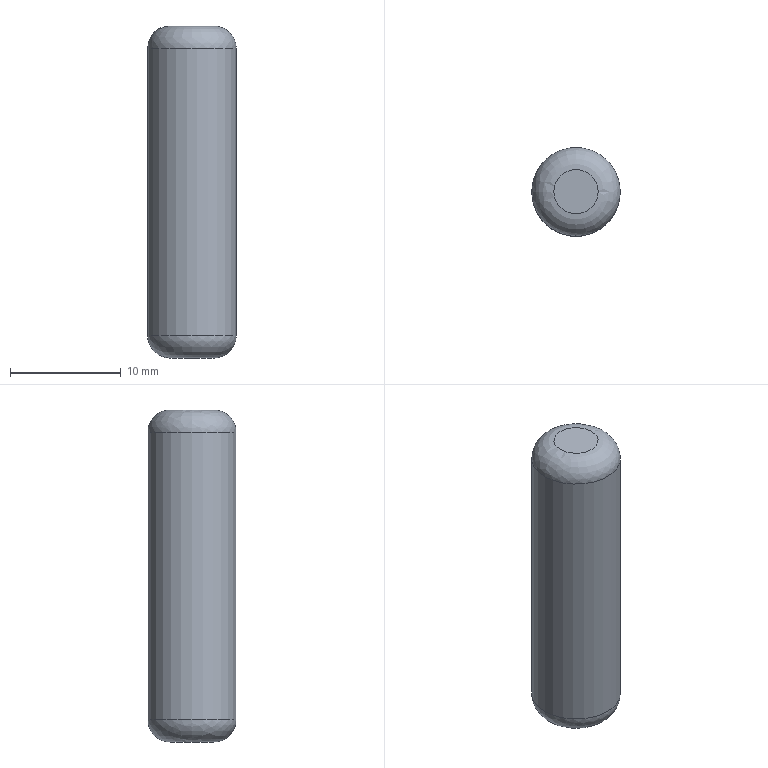Part | STEP file | Tube feed_id1762_x_t | 1 solid | 5 faces | box 8 x 8 x 30 mm | volume 1469 mm3 | plane 2 | spline 2 | cylinder 1 | commonest cylinder face diameters 8 x1
STEP:
#1=CARTESIAN_POINT('',(0.,0.,0.));
#2=DIRECTION('',(0.,0.,1.));
#3=DIRECTION('',(1.,0.,0.));
#4=AXIS2_PLACEMENT_3D('',#1,#2,#3);
#5=CARTESIAN_POINT('',(119.,82.036,-39.5));
#6=VERTEX_POINT('',#5);
#7=CARTESIAN_POINT('',(121.,82.036,-39.5));
#8=DIRECTION('',(0.,0.,-1.));
#9=DIRECTION('',(-1.,0.,0.));
#10=AXIS2_PLACEMENT_3D('',#7,#8,#9);
#11=CIRCLE('',#10,2.);
#12=CARTESIAN_POINT('',(121.,82.036,-39.5));
#13=DIRECTION('',(0.,0.,-1.));
#14=DIRECTION('',(-1.,0.,0.));
#15=AXIS2_PLACEMENT_3D('',#12,#13,#14);
#16=PLANE('',#15);
#17=CARTESIAN_POINT('',(0.,0.));
#18=DIRECTION('',(1.,0.));
#19=AXIS2_PLACEMENT_2D('',#17,#18);
#20=CIRCLE('',#19,2.);
#21=(GEOMETRIC_REPRESENTATION_CONTEXT(2)PARAMETRIC_REPRESENTATION_CONTEXT()REPRESENTATION_CONTEXT('',''));
#22=DEFINITIONAL_REPRESENTATION('',(#20),#21);
#23=PCURVE('',#16,#22);
#24=CARTESIAN_POINT('',(119.,82.036,-39.5));
#25=CARTESIAN_POINT('',(119.,86.036,-39.5));
#26=CARTESIAN_POINT('',(123.,86.036,-39.5));
#27=CARTESIAN_POINT('',(123.,82.036,-39.5));
#28=CARTESIAN_POINT('',(123.,78.036,-39.5));
#29=CARTESIAN_POINT('',(119.,78.036,-39.5));
#30=CARTESIAN_POINT('',(119.,82.036,-39.5));
#31=CARTESIAN_POINT('',(117.828,82.036,-39.5));
#32=CARTESIAN_POINT('',(117.828,88.379,-39.5));
#33=CARTESIAN_POINT('',(124.172,88.379,-39.5));
#34=CARTESIAN_POINT('',(124.172,82.036,-39.5));
#35=CARTESIAN_POINT('',(124.172,75.692,-39.5));
#36=CARTESIAN_POINT('',(117.828,75.692,-39.5));
#37=CARTESIAN_POINT('',(117.828,82.036,-39.5));
#38=CARTESIAN_POINT('',(117.,82.036,-38.672));
#39=CARTESIAN_POINT('',(117.,90.036,-38.672));
#40=CARTESIAN_POINT('',(125.,90.036,-38.672));
#41=CARTESIAN_POINT('',(125.,82.036,-38.672));
#42=CARTESIAN_POINT('',(125.,74.036,-38.672));
#43=CARTESIAN_POINT('',(117.,74.036,-38.672));
#44=CARTESIAN_POINT('',(117.,82.036,-38.672));
#45=CARTESIAN_POINT('',(117.,82.036,-37.5));
#46=CARTESIAN_POINT('',(117.,90.036,-37.5));
#47=CARTESIAN_POINT('',(125.,90.036,-37.5));
#48=CARTESIAN_POINT('',(125.,82.036,-37.5));
#49=CARTESIAN_POINT('',(125.,74.036,-37.5));
#50=CARTESIAN_POINT('',(117.,74.036,-37.5));
#51=CARTESIAN_POINT('',(117.,82.036,-37.5));
#52=(BOUNDED_SURFACE()B_SPLINE_SURFACE(3,3,((#24,#25,#26,#27,#28,#29,#30),(#31,#32,#33,#34,#35,#36,#37),(#38,#39,#40,#41,#42,#43,#44),(#45,#46,#47,#48,#49,#50,#51)),.UNSPECIFIED.,.F.,.T.,.F.)B_SPLINE_SURFACE_WITH_KNOTS((4,4),(1,3,3,3,1),(0.,1.),(-0.5,0.,0.5,1.,1.5),.UNSPECIFIED.)GEOMETRIC_REPRESENTATION_ITEM()RATIONAL_B_SPLINE_SURFACE(((1.,0.3333,0.3333,1.,0.3333,0.3333,1.),(0.8047,0.2682,0.2682,0.8047,0.2682,0.2682,0.8047),(0.8047,0.2682,0.2682,0.8047,0.2682,0.2682,0.8047),(1.,0.3333,0.3333,1.,0.3333,0.3333,1.)))REPRESENTATION_ITEM('')SURFACE());
#53=CARTESIAN_POINT('',(0.,0.));
#54=CARTESIAN_POINT('',(0.,0.02352));
#55=CARTESIAN_POINT('',(0.,0.06491));
#56=CARTESIAN_POINT('',(0.,0.1146));
#57=CARTESIAN_POINT('',(0.,0.1575));
#58=CARTESIAN_POINT('',(0.,0.196));
#59=CARTESIAN_POINT('',(0.,0.2322));
#60=CARTESIAN_POINT('',(0.,0.2678));
#61=CARTESIAN_POINT('',(0.,0.304));
#62=CARTESIAN_POINT('',(0.,0.3425));
#63=CARTESIAN_POINT('',(0.,0.3856));
#64=CARTESIAN_POINT('',(0.,0.4343));
#65=CARTESIAN_POINT('',(0.,0.5));
#66=CARTESIAN_POINT('',(0.,0.5657));
#67=CARTESIAN_POINT('',(0.,0.6144));
#68=CARTESIAN_POINT('',(0.,0.6575));
#69=CARTESIAN_POINT('',(0.,0.696));
#70=CARTESIAN_POINT('',(0.,0.7322));
#71=CARTESIAN_POINT('',(0.,0.7678));
#72=CARTESIAN_POINT('',(0.,0.804));
#73=CARTESIAN_POINT('',(0.,0.8425));
#74=CARTESIAN_POINT('',(0.,0.8854));
#75=CARTESIAN_POINT('',(0.,0.9351));
#76=CARTESIAN_POINT('',(0.,0.9765));
#77=CARTESIAN_POINT('',(0.,1.));
#78=B_SPLINE_CURVE_WITH_KNOTS('',3,(#53,#54,#55,#56,#57,#58,#59,#60,#61,#62,#63,#64,#65,#66,#67,#68,#69,#70,#71,#72,#73,#74,#75,#76,#77),.UNSPECIFIED.,.F.,.F.,(4,1,1,1,1,1,1,1,1,1,1,1,1,1,1,1,1,1,1,1,1,1,4),(0.,0.2856,0.5712,0.8568,1.142,1.428,1.714,1.999,2.285,2.57,2.856,3.142,3.427,3.713,3.998,4.284,4.57,4.855,5.141,5.426,5.712,5.998,6.283),.QUASI_UNIFORM_KNOTS.);
#79=(GEOMETRIC_REPRESENTATION_CONTEXT(2)PARAMETRIC_REPRESENTATION_CONTEXT()REPRESENTATION_CONTEXT('',''));
#80=DEFINITIONAL_REPRESENTATION('',(#78),#79);
#81=PCURVE('',#52,#80);
#82=SURFACE_CURVE('',#11,(#23,#81),.PCURVE_S1.);
#83=EDGE_CURVE('',#6,#6,#82,.T.);
#84=ORIENTED_EDGE('',*,*,#83,.T.);
#85=EDGE_LOOP('',(#84));
#86=FACE_BOUND('',#85,.T.);
#87=ADVANCED_FACE('',(#86),#16,.T.);
#88=CARTESIAN_POINT('',(117.,82.036,-11.5));
#89=VERTEX_POINT('',#88);
#90=CARTESIAN_POINT('',(121.,82.036,-11.5));
#91=DIRECTION('',(0.,0.,-1.));
#92=DIRECTION('',(-1.,0.,0.));
#93=AXIS2_PLACEMENT_3D('',#90,#91,#92);
#94=CIRCLE('',#93,4.);
#95=CARTESIAN_POINT('',(121.,82.036,-39.5));
#96=DIRECTION('',(0.,0.,1.));
#97=DIRECTION('',(1.,0.,0.));
#98=AXIS2_PLACEMENT_3D('',#95,#96,#97);
#99=CYLINDRICAL_SURFACE('',#98,4.);
#100=CARTESIAN_POINT('',(9.425,28.));
#101=DIRECTION('',(-1.,0.));
#102=VECTOR('',#101,1.);
#103=LINE('',#100,#102);
#104=(GEOMETRIC_REPRESENTATION_CONTEXT(2)PARAMETRIC_REPRESENTATION_CONTEXT()REPRESENTATION_CONTEXT('',''));
#105=DEFINITIONAL_REPRESENTATION('',(#103),#104);
#106=PCURVE('',#99,#105);
#107=CARTESIAN_POINT('',(117.,82.036,-11.5));
#108=CARTESIAN_POINT('',(117.,90.036,-11.5));
#109=CARTESIAN_POINT('',(125.,90.036,-11.5));
#110=CARTESIAN_POINT('',(125.,82.036,-11.5));
#111=CARTESIAN_POINT('',(125.,74.036,-11.5));
#112=CARTESIAN_POINT('',(117.,74.036,-11.5));
#113=CARTESIAN_POINT('',(117.,82.036,-11.5));
#114=CARTESIAN_POINT('',(117.,82.036,-10.328));
#115=CARTESIAN_POINT('',(117.,90.036,-10.328));
#116=CARTESIAN_POINT('',(125.,90.036,-10.328));
#117=CARTESIAN_POINT('',(125.,82.036,-10.328));
#118=CARTESIAN_POINT('',(125.,74.036,-10.328));
#119=CARTESIAN_POINT('',(117.,74.036,-10.328));
#120=CARTESIAN_POINT('',(117.,82.036,-10.328));
#121=CARTESIAN_POINT('',(117.828,82.036,-9.5));
#122=CARTESIAN_POINT('',(117.828,88.379,-9.5));
#123=CARTESIAN_POINT('',(124.172,88.379,-9.5));
#124=CARTESIAN_POINT('',(124.172,82.036,-9.5));
#125=CARTESIAN_POINT('',(124.172,75.692,-9.5));
#126=CARTESIAN_POINT('',(117.828,75.692,-9.5));
#127=CARTESIAN_POINT('',(117.828,82.036,-9.5));
#128=CARTESIAN_POINT('',(119.,82.036,-9.5));
#129=CARTESIAN_POINT('',(119.,86.036,-9.5));
#130=CARTESIAN_POINT('',(123.,86.036,-9.5));
#131=CARTESIAN_POINT('',(123.,82.036,-9.5));
#132=CARTESIAN_POINT('',(123.,78.036,-9.5));
#133=CARTESIAN_POINT('',(119.,78.036,-9.5));
#134=CARTESIAN_POINT('',(119.,82.036,-9.5));
#135=(BOUNDED_SURFACE()B_SPLINE_SURFACE(3,3,((#107,#108,#109,#110,#111,#112,#113),(#114,#115,#116,#117,#118,#119,#120),(#121,#122,#123,#124,#125,#126,#127),(#128,#129,#130,#131,#132,#133,#134)),.UNSPECIFIED.,.F.,.T.,.F.)B_SPLINE_SURFACE_WITH_KNOTS((4,4),(1,3,3,3,1),(0.,1.),(-0.5,0.,0.5,1.,1.5),.UNSPECIFIED.)GEOMETRIC_REPRESENTATION_ITEM()RATIONAL_B_SPLINE_SURFACE(((1.,0.3333,0.3333,1.,0.3333,0.3333,1.),(0.8047,0.2682,0.2682,0.8047,0.2682,0.2682,0.8047),(0.8047,0.2682,0.2682,0.8047,0.2682,0.2682,0.8047),(1.,0.3333,0.3333,1.,0.3333,0.3333,1.)))REPRESENTATION_ITEM('')SURFACE());
#136=CARTESIAN_POINT('',(0.,0.));
#137=CARTESIAN_POINT('',(0.,0.02352));
#138=CARTESIAN_POINT('',(0.,0.06491));
#139=CARTESIAN_POINT('',(0.,0.1146));
#140=CARTESIAN_POINT('',(0.,0.1575));
#141=CARTESIAN_POINT('',(0.,0.196));
#142=CARTESIAN_POINT('',(0.,0.2322));
#143=CARTESIAN_POINT('',(0.,0.2678));
#144=CARTESIAN_POINT('',(0.,0.304));
#145=CARTESIAN_POINT('',(0.,0.3425));
#146=CARTESIAN_POINT('',(0.,0.3856));
#147=CARTESIAN_POINT('',(0.,0.4343));
#148=CARTESIAN_POINT('',(0.,0.5));
#149=CARTESIAN_POINT('',(0.,0.5657));
#150=CARTESIAN_POINT('',(0.,0.6144));
#151=CARTESIAN_POINT('',(0.,0.6575));
#152=CARTESIAN_POINT('',(0.,0.696));
#153=CARTESIAN_POINT('',(0.,0.7322));
#154=CARTESIAN_POINT('',(0.,0.7678));
#155=CARTESIAN_POINT('',(0.,0.804));
#156=CARTESIAN_POINT('',(0.,0.8425));
#157=CARTESIAN_POINT('',(0.,0.8854));
#158=CARTESIAN_POINT('',(0.,0.9351));
#159=CARTESIAN_POINT('',(0.,0.9765));
#160=CARTESIAN_POINT('',(0.,1.));
#161=B_SPLINE_CURVE_WITH_KNOTS('',3,(#136,#137,#138,#139,#140,#141,#142,#143,#144,#145,#146,#147,#148,#149,#150,#151,#152,#153,#154,#155,#156,#157,#158,#159,#160),.UNSPECIFIED.,.F.,.F.,(4,1,1,1,1,1,1,1,1,1,1,1,1,1,1,1,1,1,1,1,1,1,4),(0.,0.2856,0.5712,0.8568,1.142,1.428,1.714,1.999,2.285,2.57,2.856,3.142,3.427,3.713,3.998,4.284,4.57,4.855,5.141,5.426,5.712,5.998,6.283),.QUASI_UNIFORM_KNOTS.);
#162=(GEOMETRIC_REPRESENTATION_CONTEXT(2)PARAMETRIC_REPRESENTATION_CONTEXT()REPRESENTATION_CONTEXT('',''));
#163=DEFINITIONAL_REPRESENTATION('',(#161),#162);
#164=PCURVE('',#135,#163);
#165=SURFACE_CURVE('',#94,(#106,#164),.PCURVE_S1.);
#166=EDGE_CURVE('',#89,#89,#165,.T.);
#167=ORIENTED_EDGE('',*,*,#166,.T.);
#168=CARTESIAN_POINT('',(117.,82.036,-37.5));
#169=VERTEX_POINT('',#168);
#170=CARTESIAN_POINT('',(117.,82.036,-37.5));
#171=CARTESIAN_POINT('',(117.,82.036,-11.5));
#172=B_SPLINE_CURVE_WITH_KNOTS('',1,(#170,#171),.UNSPECIFIED.,.F.,.F.,(2,2),(2.,28.),.PIECEWISE_BEZIER_KNOTS.);
#173=CARTESIAN_POINT('',(3.142,0.));
#174=DIRECTION('',(0.,1.));
#175=VECTOR('',#174,1.);
#176=LINE('',#173,#175);
#177=(GEOMETRIC_REPRESENTATION_CONTEXT(2)PARAMETRIC_REPRESENTATION_CONTEXT()REPRESENTATION_CONTEXT('',''));
#178=DEFINITIONAL_REPRESENTATION('',(#176),#177);
#179=PCURVE('',#99,#178);
#180=CARTESIAN_POINT('',(9.425,0.));
#181=DIRECTION('',(0.,1.));
#182=VECTOR('',#181,1.);
#183=LINE('',#180,#182);
#184=(GEOMETRIC_REPRESENTATION_CONTEXT(2)PARAMETRIC_REPRESENTATION_CONTEXT()REPRESENTATION_CONTEXT('',''));
#185=DEFINITIONAL_REPRESENTATION('',(#183),#184);
#186=PCURVE('',#99,#185);
#187=SEAM_CURVE('',#172,(#179,#186),.PCURVE_S1.);
#188=EDGE_CURVE('',#169,#89,#187,.T.);
#189=ORIENTED_EDGE('',*,*,#188,.F.);
#190=CARTESIAN_POINT('',(121.,82.036,-37.5));
#191=DIRECTION('',(0.,0.,1.));
#192=DIRECTION('',(-1.,0.,0.));
#193=AXIS2_PLACEMENT_3D('',#190,#191,#192);
#194=CIRCLE('',#193,4.);
#195=CARTESIAN_POINT('',(3.142,2.));
#196=DIRECTION('',(1.,0.));
#197=VECTOR('',#196,1.);
#198=LINE('',#195,#197);
#199=(GEOMETRIC_REPRESENTATION_CONTEXT(2)PARAMETRIC_REPRESENTATION_CONTEXT()REPRESENTATION_CONTEXT('',''));
#200=DEFINITIONAL_REPRESENTATION('',(#198),#199);
#201=PCURVE('',#99,#200);
#202=CARTESIAN_POINT('',(1.,1.));
#203=CARTESIAN_POINT('',(1.,0.9765));
#204=CARTESIAN_POINT('',(1.,0.9351));
#205=CARTESIAN_POINT('',(1.,0.8854));
#206=CARTESIAN_POINT('',(1.,0.8425));
#207=CARTESIAN_POINT('',(1.,0.804));
#208=CARTESIAN_POINT('',(1.,0.7678));
#209=CARTESIAN_POINT('',(1.,0.7322));
#210=CARTESIAN_POINT('',(1.,0.696));
#211=CARTESIAN_POINT('',(1.,0.6575));
#212=CARTESIAN_POINT('',(1.,0.6144));
#213=CARTESIAN_POINT('',(1.,0.5657));
#214=CARTESIAN_POINT('',(1.,0.5));
#215=CARTESIAN_POINT('',(1.,0.4343));
#216=CARTESIAN_POINT('',(1.,0.3856));
#217=CARTESIAN_POINT('',(1.,0.3425));
#218=CARTESIAN_POINT('',(1.,0.304));
#219=CARTESIAN_POINT('',(1.,0.2678));
#220=CARTESIAN_POINT('',(1.,0.2322));
#221=CARTESIAN_POINT('',(1.,0.196));
#222=CARTESIAN_POINT('',(1.,0.1575));
#223=CARTESIAN_POINT('',(1.,0.1146));
#224=CARTESIAN_POINT('',(1.,0.06491));
#225=CARTESIAN_POINT('',(1.,0.02352));
#226=CARTESIAN_POINT('',(1.,0.));
#227=B_SPLINE_CURVE_WITH_KNOTS('',3,(#202,#203,#204,#205,#206,#207,#208,#209,#210,#211,#212,#213,#214,#215,#216,#217,#218,#219,#220,#221,#222,#223,#224,#225,#226),.UNSPECIFIED.,.F.,.F.,(4,1,1,1,1,1,1,1,1,1,1,1,1,1,1,1,1,1,1,1,1,1,4),(0.,0.2856,0.5712,0.8568,1.142,1.428,1.714,1.999,2.285,2.57,2.856,3.142,3.427,3.713,3.998,4.284,4.57,4.855,5.141,5.426,5.712,5.998,6.283),.QUASI_UNIFORM_KNOTS.);
#228=(GEOMETRIC_REPRESENTATION_CONTEXT(2)PARAMETRIC_REPRESENTATION_CONTEXT()REPRESENTATION_CONTEXT('',''));
#229=DEFINITIONAL_REPRESENTATION('',(#227),#228);
#230=PCURVE('',#52,#229);
#231=SURFACE_CURVE('',#194,(#201,#230),.PCURVE_S1.);
#232=EDGE_CURVE('',#169,#169,#231,.T.);
#233=ORIENTED_EDGE('',*,*,#232,.T.);
#234=ORIENTED_EDGE('',*,*,#188,.T.);
#235=EDGE_LOOP('',(#167,#189,#233,#234));
#236=FACE_BOUND('',#235,.T.);
#237=ADVANCED_FACE('',(#236),#99,.T.);
#238=ORIENTED_EDGE('',*,*,#83,.F.);
#239=CARTESIAN_POINT('',(119.,82.036,-39.5));
#240=CARTESIAN_POINT('',(117.828,82.036,-39.5));
#241=CARTESIAN_POINT('',(117.,82.036,-38.672));
#242=CARTESIAN_POINT('',(117.,82.036,-37.5));
#243=(BOUNDED_CURVE()B_SPLINE_CURVE(3,(#239,#240,#241,#242),.UNSPECIFIED.,.F.,.F.)B_SPLINE_CURVE_WITH_KNOTS((4,4),(0.,1.),.PIECEWISE_BEZIER_KNOTS.)CURVE()GEOMETRIC_REPRESENTATION_ITEM()RATIONAL_B_SPLINE_CURVE((1.,0.8047,0.8047,1.))REPRESENTATION_ITEM(''));
#244=CARTESIAN_POINT('',(0.,0.));
#245=DIRECTION('',(1.,0.));
#246=VECTOR('',#245,1.);
#247=LINE('',#244,#246);
#248=(GEOMETRIC_REPRESENTATION_CONTEXT(2)PARAMETRIC_REPRESENTATION_CONTEXT()REPRESENTATION_CONTEXT('',''));
#249=DEFINITIONAL_REPRESENTATION('',(#247),#248);
#250=PCURVE('',#52,#249);
#251=CARTESIAN_POINT('',(0.,1.));
#252=DIRECTION('',(1.,0.));
#253=VECTOR('',#252,1.);
#254=LINE('',#251,#253);
#255=(GEOMETRIC_REPRESENTATION_CONTEXT(2)PARAMETRIC_REPRESENTATION_CONTEXT()REPRESENTATION_CONTEXT('',''));
#256=DEFINITIONAL_REPRESENTATION('',(#254),#255);
#257=PCURVE('',#52,#256);
#258=SEAM_CURVE('',#243,(#250,#257),.PCURVE_S1.);
#259=EDGE_CURVE('',#6,#169,#258,.T.);
#260=ORIENTED_EDGE('',*,*,#259,.T.);
#261=ORIENTED_EDGE('',*,*,#232,.F.);
#262=ORIENTED_EDGE('',*,*,#259,.F.);
#263=EDGE_LOOP('',(#238,#260,#261,#262));
#264=FACE_BOUND('',#263,.T.);
#265=ADVANCED_FACE('',(#264),#52,.T.);
#266=CARTESIAN_POINT('',(119.,82.036,-9.5));
#267=VERTEX_POINT('',#266);
#268=CARTESIAN_POINT('',(121.,82.036,-9.5));
#269=DIRECTION('',(0.,0.,1.));
#270=DIRECTION('',(-1.,0.,0.));
#271=AXIS2_PLACEMENT_3D('',#268,#269,#270);
#272=CIRCLE('',#271,2.);
#273=CARTESIAN_POINT('',(341.,-61.964,-9.5));
#274=DIRECTION('',(0.,0.,-1.));
#275=DIRECTION('',(-1.,0.,0.));
#276=AXIS2_PLACEMENT_3D('',#273,#274,#275);
#277=PLANE('',#276);
#278=CARTESIAN_POINT('',(222.,144.));
#279=CARTESIAN_POINT('',(222.,140.536));
#280=CARTESIAN_POINT('',(219.,142.268));
#281=CARTESIAN_POINT('',(216.,144.));
#282=CARTESIAN_POINT('',(219.,145.732));
#283=CARTESIAN_POINT('',(222.,147.464));
#284=CARTESIAN_POINT('',(222.,144.));
#285=(BOUNDED_CURVE()B_SPLINE_CURVE(2,(#278,#279,#280,#281,#282,#283,#284),.UNSPECIFIED.,.T.,.F.)B_SPLINE_CURVE_WITH_KNOTS((1,2,2,2,2,1),(-2.094,0.,2.094,4.189,6.283,8.378),.UNSPECIFIED.)CURVE()GEOMETRIC_REPRESENTATION_ITEM()RATIONAL_B_SPLINE_CURVE((1.,0.5,1.,0.5,1.,0.5,1.))REPRESENTATION_ITEM(''));
#286=(GEOMETRIC_REPRESENTATION_CONTEXT(2)PARAMETRIC_REPRESENTATION_CONTEXT()REPRESENTATION_CONTEXT('',''));
#287=DEFINITIONAL_REPRESENTATION('',(#285),#286);
#288=PCURVE('',#277,#287);
#289=CARTESIAN_POINT('',(1.,1.));
#290=CARTESIAN_POINT('',(1.,0.9765));
#291=CARTESIAN_POINT('',(1.,0.9351));
#292=CARTESIAN_POINT('',(1.,0.8854));
#293=CARTESIAN_POINT('',(1.,0.8425));
#294=CARTESIAN_POINT('',(1.,0.804));
#295=CARTESIAN_POINT('',(1.,0.7678));
#296=CARTESIAN_POINT('',(1.,0.7322));
#297=CARTESIAN_POINT('',(1.,0.696));
#298=CARTESIAN_POINT('',(1.,0.6575));
#299=CARTESIAN_POINT('',(1.,0.6144));
#300=CARTESIAN_POINT('',(1.,0.5657));
#301=CARTESIAN_POINT('',(1.,0.5));
#302=CARTESIAN_POINT('',(1.,0.4343));
#303=CARTESIAN_POINT('',(1.,0.3856));
#304=CARTESIAN_POINT('',(1.,0.3425));
#305=CARTESIAN_POINT('',(1.,0.304));
#306=CARTESIAN_POINT('',(1.,0.2678));
#307=CARTESIAN_POINT('',(1.,0.2322));
#308=CARTESIAN_POINT('',(1.,0.196));
#309=CARTESIAN_POINT('',(1.,0.1575));
#310=CARTESIAN_POINT('',(1.,0.1146));
#311=CARTESIAN_POINT('',(1.,0.06491));
#312=CARTESIAN_POINT('',(1.,0.02352));
#313=CARTESIAN_POINT('',(1.,0.));
#314=B_SPLINE_CURVE_WITH_KNOTS('',3,(#289,#290,#291,#292,#293,#294,#295,#296,#297,#298,#299,#300,#301,#302,#303,#304,#305,#306,#307,#308,#309,#310,#311,#312,#313),.UNSPECIFIED.,.F.,.F.,(4,1,1,1,1,1,1,1,1,1,1,1,1,1,1,1,1,1,1,1,1,1,4),(0.,0.2856,0.5712,0.8568,1.142,1.428,1.714,1.999,2.285,2.57,2.856,3.142,3.427,3.713,3.998,4.284,4.57,4.855,5.141,5.426,5.712,5.998,6.283),.QUASI_UNIFORM_KNOTS.);
#315=(GEOMETRIC_REPRESENTATION_CONTEXT(2)PARAMETRIC_REPRESENTATION_CONTEXT()REPRESENTATION_CONTEXT('',''));
#316=DEFINITIONAL_REPRESENTATION('',(#314),#315);
#317=PCURVE('',#135,#316);
#318=SURFACE_CURVE('',#272,(#288,#317),.PCURVE_S1.);
#319=EDGE_CURVE('',#267,#267,#318,.T.);
#320=ORIENTED_EDGE('',*,*,#319,.T.);
#321=EDGE_LOOP('',(#320));
#322=FACE_BOUND('',#321,.T.);
#323=ADVANCED_FACE('',(#322),#277,.F.);
#324=ORIENTED_EDGE('',*,*,#319,.F.);
#325=CARTESIAN_POINT('',(117.,82.036,-11.5));
#326=CARTESIAN_POINT('',(117.,82.036,-10.328));
#327=CARTESIAN_POINT('',(117.828,82.036,-9.5));
#328=CARTESIAN_POINT('',(119.,82.036,-9.5));
#329=(BOUNDED_CURVE()B_SPLINE_CURVE(3,(#325,#326,#327,#328),.UNSPECIFIED.,.F.,.F.)B_SPLINE_CURVE_WITH_KNOTS((4,4),(0.,1.),.PIECEWISE_BEZIER_KNOTS.)CURVE()GEOMETRIC_REPRESENTATION_ITEM()RATIONAL_B_SPLINE_CURVE((1.,0.8047,0.8047,1.))REPRESENTATION_ITEM(''));
#330=CARTESIAN_POINT('',(0.,1.));
#331=DIRECTION('',(1.,0.));
#332=VECTOR('',#331,1.);
#333=LINE('',#330,#332);
#334=(GEOMETRIC_REPRESENTATION_CONTEXT(2)PARAMETRIC_REPRESENTATION_CONTEXT()REPRESENTATION_CONTEXT('',''));
#335=DEFINITIONAL_REPRESENTATION('',(#333),#334);
#336=PCURVE('',#135,#335);
#337=CARTESIAN_POINT('',(0.,0.));
#338=DIRECTION('',(1.,0.));
#339=VECTOR('',#338,1.);
#340=LINE('',#337,#339);
#341=(GEOMETRIC_REPRESENTATION_CONTEXT(2)PARAMETRIC_REPRESENTATION_CONTEXT()REPRESENTATION_CONTEXT('',''));
#342=DEFINITIONAL_REPRESENTATION('',(#340),#341);
#343=PCURVE('',#135,#342);
#344=SEAM_CURVE('',#329,(#336,#343),.PCURVE_S1.);
#345=EDGE_CURVE('',#89,#267,#344,.T.);
#346=ORIENTED_EDGE('',*,*,#345,.F.);
#347=ORIENTED_EDGE('',*,*,#166,.F.);
#348=ORIENTED_EDGE('',*,*,#345,.T.);
#349=EDGE_LOOP('',(#324,#346,#347,#348));
#350=FACE_BOUND('',#349,.T.);
#351=ADVANCED_FACE('',(#350),#135,.T.);
#352=CLOSED_SHELL('',(#87,#237,#265,#323,#351));
#353=MANIFOLD_SOLID_BREP('',#352);
#354=(LENGTH_UNIT()NAMED_UNIT(*)SI_UNIT(.MILLI.,.METRE.));
#355=UNCERTAINTY_MEASURE_WITH_UNIT(LENGTH_MEASURE(0.00001),#354,'','');
#356=(NAMED_UNIT(*)PLANE_ANGLE_UNIT()SI_UNIT($,.RADIAN.));
#357=(NAMED_UNIT(*)SI_UNIT($,.STERADIAN.)SOLID_ANGLE_UNIT());
#358=(GEOMETRIC_REPRESENTATION_CONTEXT(3)GLOBAL_UNCERTAINTY_ASSIGNED_CONTEXT((#355))GLOBAL_UNIT_ASSIGNED_CONTEXT((#354,#356,#357))REPRESENTATION_CONTEXT('',''));
#359=ADVANCED_BREP_SHAPE_REPRESENTATION('',(#4,#353),#358);